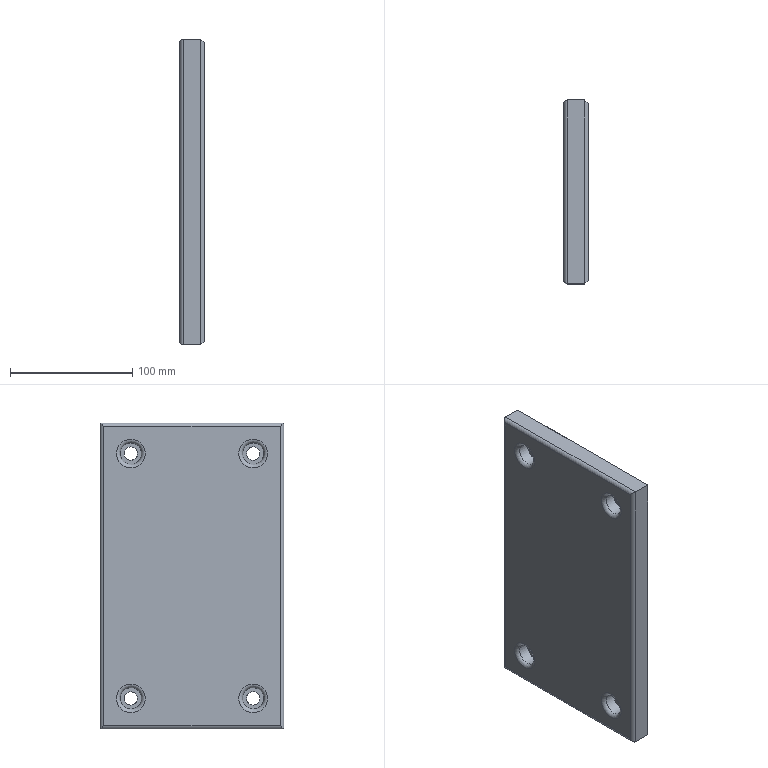Part | NX | features MAIN_BODY 2 | 1 solid | 30 faces | box 20 x 150 x 250 mm | volume 729858 mm3 | plane 14 | cylinder 12 | torus 4 | commonest cylinder face diameters 6 x4 11 x4 17.5 x4
STEP:
#1=CARTESIAN_POINT('',(-1150.,-208.,32.));
#2=VERTEX_POINT('',#1);
#3=CARTESIAN_POINT('',(-1150.,-208.,-212.));
#4=VERTEX_POINT('',#3);
#5=CARTESIAN_POINT('',(-1150.,-208.,-215.));
#6=DIRECTION('',(0.,0.,1.));
#7=VECTOR('',#6,1000.);
#8=LINE('',#5,#7);
#9=EDGE_CURVE('',#2,#4,#8,.F.);
#10=ORIENTED_EDGE('',*,*,#9,.T.);
#11=CARTESIAN_POINT('',(-1150.,-352.,-212.));
#12=VERTEX_POINT('',#11);
#13=CARTESIAN_POINT('',(-1150.,-355.,-212.));
#14=DIRECTION('',(0.,1.,0.));
#15=VECTOR('',#14,1000.);
#16=LINE('',#13,#15);
#17=EDGE_CURVE('',#4,#12,#16,.F.);
#18=ORIENTED_EDGE('',*,*,#17,.T.);
#19=CARTESIAN_POINT('',(-1150.,-352.,32.));
#20=VERTEX_POINT('',#19);
#21=CARTESIAN_POINT('',(-1150.,-352.,35.));
#22=DIRECTION('',(0.,0.,-1.));
#23=VECTOR('',#22,1000.);
#24=LINE('',#21,#23);
#25=EDGE_CURVE('',#12,#20,#24,.F.);
#26=ORIENTED_EDGE('',*,*,#25,.T.);
#27=CARTESIAN_POINT('',(-1150.,-205.,32.));
#28=DIRECTION('',(0.,-1.,0.));
#29=VECTOR('',#28,1000.);
#30=LINE('',#27,#29);
#31=EDGE_CURVE('',#20,#2,#30,.F.);
#32=ORIENTED_EDGE('',*,*,#31,.T.);
#33=EDGE_LOOP('',(#10,#18,#26,#32));
#34=FACE_BOUND('',#33,.T.);
#35=CARTESIAN_POINT('',(-1150.,-230.,-178.25));
#36=VERTEX_POINT('',#35);
#37=CARTESIAN_POINT('',(-1150.,-230.,-190.));
#38=DIRECTION('',(1.,0.,0.));
#39=DIRECTION('',(0.,0.,1.));
#40=AXIS2_PLACEMENT_3D('',#37,#38,#39);
#41=CIRCLE('',#40,11.75);
#42=EDGE_CURVE('',#36,#36,#41,.T.);
#43=ORIENTED_EDGE('',*,*,#42,.T.);
#44=EDGE_LOOP('',(#43));
#45=FACE_BOUND('',#44,.T.);
#46=CARTESIAN_POINT('',(-1150.,-330.,-178.25));
#47=VERTEX_POINT('',#46);
#48=CARTESIAN_POINT('',(-1150.,-330.,-190.));
#49=DIRECTION('',(1.,0.,0.));
#50=DIRECTION('',(0.,0.,1.));
#51=AXIS2_PLACEMENT_3D('',#48,#49,#50);
#52=CIRCLE('',#51,11.75);
#53=EDGE_CURVE('',#47,#47,#52,.T.);
#54=ORIENTED_EDGE('',*,*,#53,.T.);
#55=EDGE_LOOP('',(#54));
#56=FACE_BOUND('',#55,.T.);
#57=CARTESIAN_POINT('',(-1150.,-330.,21.75));
#58=VERTEX_POINT('',#57);
#59=CARTESIAN_POINT('',(-1150.,-330.,10.));
#60=DIRECTION('',(1.,0.,0.));
#61=DIRECTION('',(0.,0.,1.));
#62=AXIS2_PLACEMENT_3D('',#59,#60,#61);
#63=CIRCLE('',#62,11.75);
#64=EDGE_CURVE('',#58,#58,#63,.T.);
#65=ORIENTED_EDGE('',*,*,#64,.T.);
#66=EDGE_LOOP('',(#65));
#67=FACE_BOUND('',#66,.T.);
#68=CARTESIAN_POINT('',(-1150.,-230.,21.75));
#69=VERTEX_POINT('',#68);
#70=CARTESIAN_POINT('',(-1150.,-230.,10.));
#71=DIRECTION('',(1.,0.,0.));
#72=DIRECTION('',(0.,0.,1.));
#73=AXIS2_PLACEMENT_3D('',#70,#71,#72);
#74=CIRCLE('',#73,11.75);
#75=EDGE_CURVE('',#69,#69,#74,.T.);
#76=ORIENTED_EDGE('',*,*,#75,.T.);
#77=EDGE_LOOP('',(#76));
#78=FACE_BOUND('',#77,.T.);
#79=CARTESIAN_POINT('',(-1150.,-205.,35.));
#80=DIRECTION('',(1.,0.,0.));
#81=DIRECTION('',(0.,0.,1.));
#82=AXIS2_PLACEMENT_3D('',#79,#80,#81);
#83=PLANE('',#82);
#84=ADVANCED_FACE('',(#34,#45,#56,#67,#78),#83,.F.);
#85=CARTESIAN_POINT('',(-1130.,-324.5,10.));
#86=VERTEX_POINT('',#85);
#87=CARTESIAN_POINT('',(-1130.,-330.,10.));
#88=DIRECTION('',(-1.,0.,0.));
#89=DIRECTION('',(0.,1.,0.));
#90=AXIS2_PLACEMENT_3D('',#87,#88,#89);
#91=CIRCLE('',#90,5.5);
#92=EDGE_CURVE('',#86,#86,#91,.T.);
#93=ORIENTED_EDGE('',*,*,#92,.F.);
#94=EDGE_LOOP('',(#93));
#95=FACE_BOUND('',#94,.T.);
#96=CARTESIAN_POINT('',(-1138.,-330.,4.5));
#97=VERTEX_POINT('',#96);
#98=CARTESIAN_POINT('',(-1138.,-330.,10.));
#99=DIRECTION('',(-1.,0.,0.));
#100=DIRECTION('',(0.,0.,-1.));
#101=AXIS2_PLACEMENT_3D('',#98,#99,#100);
#102=CIRCLE('',#101,5.5);
#103=EDGE_CURVE('',#97,#97,#102,.T.);
#104=ORIENTED_EDGE('',*,*,#103,.T.);
#105=EDGE_LOOP('',(#104));
#106=FACE_BOUND('',#105,.T.);
#107=CARTESIAN_POINT('',(-1150.,-330.,10.));
#108=DIRECTION('',(1.,0.,0.));
#109=DIRECTION('',(0.,0.,1.));
#110=AXIS2_PLACEMENT_3D('',#107,#108,#109);
#111=CYLINDRICAL_SURFACE('',#110,5.5);
#112=ADVANCED_FACE('',(#95,#106),#111,.F.);
#113=CARTESIAN_POINT('',(-1130.,-235.5,-190.));
#114=VERTEX_POINT('',#113);
#115=CARTESIAN_POINT('',(-1130.,-230.,-190.));
#116=DIRECTION('',(-1.,0.,0.));
#117=DIRECTION('',(0.,-1.,0.));
#118=AXIS2_PLACEMENT_3D('',#115,#116,#117);
#119=CIRCLE('',#118,5.5);
#120=EDGE_CURVE('',#114,#114,#119,.T.);
#121=ORIENTED_EDGE('',*,*,#120,.F.);
#122=EDGE_LOOP('',(#121));
#123=FACE_BOUND('',#122,.T.);
#124=CARTESIAN_POINT('',(-1138.,-230.,-195.5));
#125=VERTEX_POINT('',#124);
#126=CARTESIAN_POINT('',(-1138.,-230.,-190.));
#127=DIRECTION('',(-1.,0.,0.));
#128=DIRECTION('',(0.,0.,-1.));
#129=AXIS2_PLACEMENT_3D('',#126,#127,#128);
#130=CIRCLE('',#129,5.5);
#131=EDGE_CURVE('',#125,#125,#130,.T.);
#132=ORIENTED_EDGE('',*,*,#131,.T.);
#133=EDGE_LOOP('',(#132));
#134=FACE_BOUND('',#133,.T.);
#135=CARTESIAN_POINT('',(-1150.,-230.,-190.));
#136=DIRECTION('',(1.,0.,0.));
#137=DIRECTION('',(0.,0.,1.));
#138=AXIS2_PLACEMENT_3D('',#135,#136,#137);
#139=CYLINDRICAL_SURFACE('',#138,5.5);
#140=ADVANCED_FACE('',(#123,#134),#139,.F.);
#141=CARTESIAN_POINT('',(-1130.,-352.,32.));
#142=VERTEX_POINT('',#141);
#143=CARTESIAN_POINT('',(-1130.,-352.,-212.));
#144=VERTEX_POINT('',#143);
#145=CARTESIAN_POINT('',(-1130.,-352.,35.));
#146=DIRECTION('',(0.,0.,-1.));
#147=VECTOR('',#146,1000.);
#148=LINE('',#145,#147);
#149=EDGE_CURVE('',#142,#144,#148,.T.);
#150=ORIENTED_EDGE('',*,*,#149,.T.);
#151=CARTESIAN_POINT('',(-1130.,-208.,-212.));
#152=VERTEX_POINT('',#151);
#153=CARTESIAN_POINT('',(-1130.,-205.,-212.));
#154=DIRECTION('',(0.,1.,0.));
#155=VECTOR('',#154,1000.);
#156=LINE('',#153,#155);
#157=EDGE_CURVE('',#144,#152,#156,.T.);
#158=ORIENTED_EDGE('',*,*,#157,.T.);
#159=CARTESIAN_POINT('',(-1130.,-208.,32.));
#160=VERTEX_POINT('',#159);
#161=CARTESIAN_POINT('',(-1130.,-208.,35.));
#162=DIRECTION('',(0.,0.,1.));
#163=VECTOR('',#162,1000.);
#164=LINE('',#161,#163);
#165=EDGE_CURVE('',#152,#160,#164,.T.);
#166=ORIENTED_EDGE('',*,*,#165,.T.);
#167=CARTESIAN_POINT('',(-1130.,-205.,32.));
#168=DIRECTION('',(0.,-1.,0.));
#169=VECTOR('',#168,1000.);
#170=LINE('',#167,#169);
#171=EDGE_CURVE('',#160,#142,#170,.T.);
#172=ORIENTED_EDGE('',*,*,#171,.T.);
#173=EDGE_LOOP('',(#150,#158,#166,#172));
#174=FACE_BOUND('',#173,.T.);
#175=CARTESIAN_POINT('',(-1130.,-235.5,10.));
#176=VERTEX_POINT('',#175);
#177=CARTESIAN_POINT('',(-1130.,-230.,10.));
#178=DIRECTION('',(1.,0.,0.));
#179=DIRECTION('',(0.,-1.,0.));
#180=AXIS2_PLACEMENT_3D('',#177,#178,#179);
#181=CIRCLE('',#180,5.5);
#182=EDGE_CURVE('',#176,#176,#181,.T.);
#183=ORIENTED_EDGE('',*,*,#182,.F.);
#184=EDGE_LOOP('',(#183));
#185=FACE_BOUND('',#184,.T.);
#186=ORIENTED_EDGE('',*,*,#92,.T.);
#187=EDGE_LOOP('',(#186));
#188=FACE_BOUND('',#187,.T.);
#189=CARTESIAN_POINT('',(-1130.,-324.5,-190.));
#190=VERTEX_POINT('',#189);
#191=CARTESIAN_POINT('',(-1130.,-330.,-190.));
#192=DIRECTION('',(1.,0.,0.));
#193=DIRECTION('',(0.,1.,0.));
#194=AXIS2_PLACEMENT_3D('',#191,#192,#193);
#195=CIRCLE('',#194,5.5);
#196=EDGE_CURVE('',#190,#190,#195,.T.);
#197=ORIENTED_EDGE('',*,*,#196,.F.);
#198=EDGE_LOOP('',(#197));
#199=FACE_BOUND('',#198,.T.);
#200=ORIENTED_EDGE('',*,*,#120,.T.);
#201=EDGE_LOOP('',(#200));
#202=FACE_BOUND('',#201,.T.);
#203=CARTESIAN_POINT('',(-1130.,-205.,35.));
#204=DIRECTION('',(1.,0.,0.));
#205=DIRECTION('',(0.,0.,1.));
#206=AXIS2_PLACEMENT_3D('',#203,#204,#205);
#207=PLANE('',#206);
#208=ADVANCED_FACE('',(#174,#185,#188,#199,#202),#207,.T.);
#209=CARTESIAN_POINT('',(-1147.,-205.,35.));
#210=VERTEX_POINT('',#209);
#211=CARTESIAN_POINT('',(-1133.,-205.,35.));
#212=VERTEX_POINT('',#211);
#213=CARTESIAN_POINT('',(-1150.,-205.,35.));
#214=DIRECTION('',(1.,0.,0.));
#215=VECTOR('',#214,1000.);
#216=LINE('',#213,#215);
#217=EDGE_CURVE('',#210,#212,#216,.T.);
#218=ORIENTED_EDGE('',*,*,#217,.T.);
#219=CARTESIAN_POINT('',(-1133.,-205.,-215.));
#220=VERTEX_POINT('',#219);
#221=CARTESIAN_POINT('',(-1133.,-205.,-215.));
#222=DIRECTION('',(0.,0.,-1.));
#223=VECTOR('',#222,1000.);
#224=LINE('',#221,#223);
#225=EDGE_CURVE('',#212,#220,#224,.T.);
#226=ORIENTED_EDGE('',*,*,#225,.T.);
#227=CARTESIAN_POINT('',(-1147.,-205.,-215.));
#228=VERTEX_POINT('',#227);
#229=CARTESIAN_POINT('',(-1150.,-205.,-215.));
#230=DIRECTION('',(1.,0.,0.));
#231=VECTOR('',#230,1000.);
#232=LINE('',#229,#231);
#233=EDGE_CURVE('',#228,#220,#232,.T.);
#234=ORIENTED_EDGE('',*,*,#233,.F.);
#235=CARTESIAN_POINT('',(-1147.,-205.,35.));
#236=DIRECTION('',(0.,0.,1.));
#237=VECTOR('',#236,1000.);
#238=LINE('',#235,#237);
#239=EDGE_CURVE('',#228,#210,#238,.T.);
#240=ORIENTED_EDGE('',*,*,#239,.T.);
#241=EDGE_LOOP('',(#218,#226,#234,#240));
#242=FACE_BOUND('',#241,.T.);
#243=CARTESIAN_POINT('',(-1150.,-205.,-215.));
#244=DIRECTION('',(0.,1.,0.));
#245=DIRECTION('',(0.,0.,-1.));
#246=AXIS2_PLACEMENT_3D('',#243,#244,#245);
#247=PLANE('',#246);
#248=ADVANCED_FACE('',(#242),#247,.T.);
#249=CARTESIAN_POINT('',(-1147.,-355.,35.));
#250=VERTEX_POINT('',#249);
#251=CARTESIAN_POINT('',(-1133.,-355.,35.));
#252=VERTEX_POINT('',#251);
#253=CARTESIAN_POINT('',(-1150.,-355.,35.));
#254=DIRECTION('',(1.,0.,0.));
#255=VECTOR('',#254,1000.);
#256=LINE('',#253,#255);
#257=EDGE_CURVE('',#250,#252,#256,.T.);
#258=ORIENTED_EDGE('',*,*,#257,.T.);
#259=CARTESIAN_POINT('',(-1133.,-205.,35.));
#260=DIRECTION('',(0.,1.,0.));
#261=VECTOR('',#260,1000.);
#262=LINE('',#259,#261);
#263=EDGE_CURVE('',#252,#212,#262,.T.);
#264=ORIENTED_EDGE('',*,*,#263,.T.);
#265=ORIENTED_EDGE('',*,*,#217,.F.);
#266=CARTESIAN_POINT('',(-1147.,-355.,35.));
#267=DIRECTION('',(0.,-1.,0.));
#268=VECTOR('',#267,1000.);
#269=LINE('',#266,#268);
#270=EDGE_CURVE('',#210,#250,#269,.T.);
#271=ORIENTED_EDGE('',*,*,#270,.T.);
#272=EDGE_LOOP('',(#258,#264,#265,#271));
#273=FACE_BOUND('',#272,.T.);
#274=CARTESIAN_POINT('',(-1150.,-205.,35.));
#275=DIRECTION('',(0.,0.,1.));
#276=DIRECTION('',(0.,1.,0.));
#277=AXIS2_PLACEMENT_3D('',#274,#275,#276);
#278=PLANE('',#277);
#279=ADVANCED_FACE('',(#273),#278,.T.);
#280=CARTESIAN_POINT('',(-1147.,-355.,-215.));
#281=VERTEX_POINT('',#280);
#282=CARTESIAN_POINT('',(-1133.,-355.,-215.));
#283=VERTEX_POINT('',#282);
#284=CARTESIAN_POINT('',(-1150.,-355.,-215.));
#285=DIRECTION('',(1.,0.,0.));
#286=VECTOR('',#285,1000.);
#287=LINE('',#284,#286);
#288=EDGE_CURVE('',#281,#283,#287,.T.);
#289=ORIENTED_EDGE('',*,*,#288,.T.);
#290=CARTESIAN_POINT('',(-1133.,-355.,35.));
#291=DIRECTION('',(0.,0.,1.));
#292=VECTOR('',#291,1000.);
#293=LINE('',#290,#292);
#294=EDGE_CURVE('',#283,#252,#293,.T.);
#295=ORIENTED_EDGE('',*,*,#294,.T.);
#296=ORIENTED_EDGE('',*,*,#257,.F.);
#297=CARTESIAN_POINT('',(-1147.,-355.,-215.));
#298=DIRECTION('',(0.,0.,-1.));
#299=VECTOR('',#298,1000.);
#300=LINE('',#297,#299);
#301=EDGE_CURVE('',#250,#281,#300,.T.);
#302=ORIENTED_EDGE('',*,*,#301,.T.);
#303=EDGE_LOOP('',(#289,#295,#296,#302));
#304=FACE_BOUND('',#303,.T.);
#305=CARTESIAN_POINT('',(-1150.,-355.,35.));
#306=DIRECTION('',(0.,-1.,0.));
#307=DIRECTION('',(0.,0.,1.));
#308=AXIS2_PLACEMENT_3D('',#305,#306,#307);
#309=PLANE('',#308);
#310=ADVANCED_FACE('',(#304),#309,.T.);
#311=ORIENTED_EDGE('',*,*,#233,.T.);
#312=CARTESIAN_POINT('',(-1133.,-355.,-215.));
#313=DIRECTION('',(0.,-1.,0.));
#314=VECTOR('',#313,1000.);
#315=LINE('',#312,#314);
#316=EDGE_CURVE('',#220,#283,#315,.T.);
#317=ORIENTED_EDGE('',*,*,#316,.T.);
#318=ORIENTED_EDGE('',*,*,#288,.F.);
#319=CARTESIAN_POINT('',(-1147.,-205.,-215.));
#320=DIRECTION('',(0.,1.,0.));
#321=VECTOR('',#320,1000.);
#322=LINE('',#319,#321);
#323=EDGE_CURVE('',#281,#228,#322,.T.);
#324=ORIENTED_EDGE('',*,*,#323,.T.);
#325=EDGE_LOOP('',(#311,#317,#318,#324));
#326=FACE_BOUND('',#325,.T.);
#327=CARTESIAN_POINT('',(-1150.,-355.,-215.));
#328=DIRECTION('',(0.,0.,-1.));
#329=DIRECTION('',(0.,-1.,0.));
#330=AXIS2_PLACEMENT_3D('',#327,#328,#329);
#331=PLANE('',#330);
#332=ADVANCED_FACE('',(#326),#331,.T.);
#333=CARTESIAN_POINT('',(-1138.,-330.,-184.5));
#334=VERTEX_POINT('',#333);
#335=CARTESIAN_POINT('',(-1138.,-330.,-190.));
#336=DIRECTION('',(1.,0.,0.));
#337=DIRECTION('',(0.,0.,1.));
#338=AXIS2_PLACEMENT_3D('',#335,#336,#337);
#339=CIRCLE('',#338,5.5);
#340=EDGE_CURVE('',#334,#334,#339,.F.);
#341=ORIENTED_EDGE('',*,*,#340,.T.);
#342=EDGE_LOOP('',(#341));
#343=FACE_BOUND('',#342,.T.);
#344=ORIENTED_EDGE('',*,*,#196,.T.);
#345=EDGE_LOOP('',(#344));
#346=FACE_BOUND('',#345,.T.);
#347=CARTESIAN_POINT('',(-1150.,-330.,-190.));
#348=DIRECTION('',(1.,0.,0.));
#349=DIRECTION('',(0.,0.,1.));
#350=AXIS2_PLACEMENT_3D('',#347,#348,#349);
#351=CYLINDRICAL_SURFACE('',#350,5.5);
#352=ADVANCED_FACE('',(#343,#346),#351,.F.);
#353=CARTESIAN_POINT('',(-1138.,-230.,15.5));
#354=VERTEX_POINT('',#353);
#355=CARTESIAN_POINT('',(-1138.,-230.,10.));
#356=DIRECTION('',(1.,0.,0.));
#357=DIRECTION('',(0.,0.,1.));
#358=AXIS2_PLACEMENT_3D('',#355,#356,#357);
#359=CIRCLE('',#358,5.5);
#360=EDGE_CURVE('',#354,#354,#359,.F.);
#361=ORIENTED_EDGE('',*,*,#360,.T.);
#362=EDGE_LOOP('',(#361));
#363=FACE_BOUND('',#362,.T.);
#364=ORIENTED_EDGE('',*,*,#182,.T.);
#365=EDGE_LOOP('',(#364));
#366=FACE_BOUND('',#365,.T.);
#367=CARTESIAN_POINT('',(-1150.,-230.,10.));
#368=DIRECTION('',(1.,0.,0.));
#369=DIRECTION('',(0.,0.,1.));
#370=AXIS2_PLACEMENT_3D('',#367,#368,#369);
#371=CYLINDRICAL_SURFACE('',#370,5.5);
#372=ADVANCED_FACE('',(#363,#366),#371,.F.);
#373=CARTESIAN_POINT('',(-1147.,-230.,-181.25));
#374=VERTEX_POINT('',#373);
#375=CARTESIAN_POINT('',(-1147.,-230.,-190.));
#376=DIRECTION('',(1.,0.,0.));
#377=DIRECTION('',(0.,0.,1.));
#378=AXIS2_PLACEMENT_3D('',#375,#376,#377);
#379=CIRCLE('',#378,8.75);
#380=EDGE_CURVE('',#374,#374,#379,.F.);
#381=ORIENTED_EDGE('',*,*,#380,.T.);
#382=EDGE_LOOP('',(#381));
#383=FACE_BOUND('',#382,.T.);
#384=CARTESIAN_POINT('',(-1138.,-238.75,-190.));
#385=VERTEX_POINT('',#384);
#386=CARTESIAN_POINT('',(-1138.,-230.,-190.));
#387=DIRECTION('',(-1.,0.,0.));
#388=DIRECTION('',(0.,-1.,0.));
#389=AXIS2_PLACEMENT_3D('',#386,#387,#388);
#390=CIRCLE('',#389,8.75);
#391=EDGE_CURVE('',#385,#385,#390,.T.);
#392=ORIENTED_EDGE('',*,*,#391,.F.);
#393=EDGE_LOOP('',(#392));
#394=FACE_BOUND('',#393,.T.);
#395=CARTESIAN_POINT('',(-1160.,-230.,-190.));
#396=DIRECTION('',(1.,0.,0.));
#397=DIRECTION('',(0.,0.,1.));
#398=AXIS2_PLACEMENT_3D('',#395,#396,#397);
#399=CYLINDRICAL_SURFACE('',#398,8.75);
#400=ADVANCED_FACE('',(#383,#394),#399,.F.);
#401=ORIENTED_EDGE('',*,*,#131,.F.);
#402=EDGE_LOOP('',(#401));
#403=FACE_BOUND('',#402,.T.);
#404=ORIENTED_EDGE('',*,*,#391,.T.);
#405=EDGE_LOOP('',(#404));
#406=FACE_BOUND('',#405,.T.);
#407=CARTESIAN_POINT('',(-1138.,-230.,-190.));
#408=DIRECTION('',(-1.,0.,0.));
#409=DIRECTION('',(0.,0.,-1.));
#410=AXIS2_PLACEMENT_3D('',#407,#408,#409);
#411=PLANE('',#410);
#412=ADVANCED_FACE('',(#403,#406),#411,.T.);
#413=CARTESIAN_POINT('',(-1147.,-230.,18.75));
#414=VERTEX_POINT('',#413);
#415=CARTESIAN_POINT('',(-1147.,-230.,10.));
#416=DIRECTION('',(1.,0.,0.));
#417=DIRECTION('',(0.,0.,1.));
#418=AXIS2_PLACEMENT_3D('',#415,#416,#417);
#419=CIRCLE('',#418,8.75);
#420=EDGE_CURVE('',#414,#414,#419,.F.);
#421=ORIENTED_EDGE('',*,*,#420,.T.);
#422=EDGE_LOOP('',(#421));
#423=FACE_BOUND('',#422,.T.);
#424=CARTESIAN_POINT('',(-1138.,-238.75,10.));
#425=VERTEX_POINT('',#424);
#426=CARTESIAN_POINT('',(-1138.,-230.,10.));
#427=DIRECTION('',(1.,0.,0.));
#428=DIRECTION('',(0.,-1.,0.));
#429=AXIS2_PLACEMENT_3D('',#426,#427,#428);
#430=CIRCLE('',#429,8.75);
#431=EDGE_CURVE('',#425,#425,#430,.T.);
#432=ORIENTED_EDGE('',*,*,#431,.T.);
#433=EDGE_LOOP('',(#432));
#434=FACE_BOUND('',#433,.T.);
#435=CARTESIAN_POINT('',(-1160.,-230.,10.));
#436=DIRECTION('',(1.,0.,0.));
#437=DIRECTION('',(0.,0.,1.));
#438=AXIS2_PLACEMENT_3D('',#435,#436,#437);
#439=CYLINDRICAL_SURFACE('',#438,8.75);
#440=ADVANCED_FACE('',(#423,#434),#439,.F.);
#441=ORIENTED_EDGE('',*,*,#431,.F.);
#442=EDGE_LOOP('',(#441));
#443=FACE_BOUND('',#442,.T.);
#444=ORIENTED_EDGE('',*,*,#360,.F.);
#445=EDGE_LOOP('',(#444));
#446=FACE_BOUND('',#445,.T.);
#447=CARTESIAN_POINT('',(-1138.,-230.,10.));
#448=DIRECTION('',(1.,0.,0.));
#449=DIRECTION('',(0.,0.,1.));
#450=AXIS2_PLACEMENT_3D('',#447,#448,#449);
#451=PLANE('',#450);
#452=ADVANCED_FACE('',(#443,#446),#451,.F.);
#453=CARTESIAN_POINT('',(-1147.,-330.,-181.25));
#454=VERTEX_POINT('',#453);
#455=CARTESIAN_POINT('',(-1147.,-330.,-190.));
#456=DIRECTION('',(1.,0.,0.));
#457=DIRECTION('',(0.,0.,1.));
#458=AXIS2_PLACEMENT_3D('',#455,#456,#457);
#459=CIRCLE('',#458,8.75);
#460=EDGE_CURVE('',#454,#454,#459,.F.);
#461=ORIENTED_EDGE('',*,*,#460,.T.);
#462=EDGE_LOOP('',(#461));
#463=FACE_BOUND('',#462,.T.);
#464=CARTESIAN_POINT('',(-1138.,-321.25,-190.));
#465=VERTEX_POINT('',#464);
#466=CARTESIAN_POINT('',(-1138.,-330.,-190.));
#467=DIRECTION('',(1.,0.,0.));
#468=DIRECTION('',(0.,1.,0.));
#469=AXIS2_PLACEMENT_3D('',#466,#467,#468);
#470=CIRCLE('',#469,8.75);
#471=EDGE_CURVE('',#465,#465,#470,.T.);
#472=ORIENTED_EDGE('',*,*,#471,.T.);
#473=EDGE_LOOP('',(#472));
#474=FACE_BOUND('',#473,.T.);
#475=CARTESIAN_POINT('',(-1160.,-330.,-190.));
#476=DIRECTION('',(1.,0.,0.));
#477=DIRECTION('',(0.,0.,1.));
#478=AXIS2_PLACEMENT_3D('',#475,#476,#477);
#479=CYLINDRICAL_SURFACE('',#478,8.75);
#480=ADVANCED_FACE('',(#463,#474),#479,.F.);
#481=ORIENTED_EDGE('',*,*,#471,.F.);
#482=EDGE_LOOP('',(#481));
#483=FACE_BOUND('',#482,.T.);
#484=ORIENTED_EDGE('',*,*,#340,.F.);
#485=EDGE_LOOP('',(#484));
#486=FACE_BOUND('',#485,.T.);
#487=CARTESIAN_POINT('',(-1138.,-330.,-190.));
#488=DIRECTION('',(1.,0.,0.));
#489=DIRECTION('',(0.,0.,1.));
#490=AXIS2_PLACEMENT_3D('',#487,#488,#489);
#491=PLANE('',#490);
#492=ADVANCED_FACE('',(#483,#486),#491,.F.);
#493=CARTESIAN_POINT('',(-1147.,-330.,18.75));
#494=VERTEX_POINT('',#493);
#495=CARTESIAN_POINT('',(-1147.,-330.,10.));
#496=DIRECTION('',(1.,0.,0.));
#497=DIRECTION('',(0.,0.,1.));
#498=AXIS2_PLACEMENT_3D('',#495,#496,#497);
#499=CIRCLE('',#498,8.75);
#500=EDGE_CURVE('',#494,#494,#499,.F.);
#501=ORIENTED_EDGE('',*,*,#500,.T.);
#502=EDGE_LOOP('',(#501));
#503=FACE_BOUND('',#502,.T.);
#504=CARTESIAN_POINT('',(-1138.,-321.25,10.));
#505=VERTEX_POINT('',#504);
#506=CARTESIAN_POINT('',(-1138.,-330.,10.));
#507=DIRECTION('',(-1.,0.,0.));
#508=DIRECTION('',(0.,1.,0.));
#509=AXIS2_PLACEMENT_3D('',#506,#507,#508);
#510=CIRCLE('',#509,8.75);
#511=EDGE_CURVE('',#505,#505,#510,.T.);
#512=ORIENTED_EDGE('',*,*,#511,.F.);
#513=EDGE_LOOP('',(#512));
#514=FACE_BOUND('',#513,.T.);
#515=CARTESIAN_POINT('',(-1160.,-330.,10.));
#516=DIRECTION('',(1.,0.,0.));
#517=DIRECTION('',(0.,0.,1.));
#518=AXIS2_PLACEMENT_3D('',#515,#516,#517);
#519=CYLINDRICAL_SURFACE('',#518,8.75);
#520=ADVANCED_FACE('',(#503,#514),#519,.F.);
#521=ORIENTED_EDGE('',*,*,#103,.F.);
#522=EDGE_LOOP('',(#521));
#523=FACE_BOUND('',#522,.T.);
#524=ORIENTED_EDGE('',*,*,#511,.T.);
#525=EDGE_LOOP('',(#524));
#526=FACE_BOUND('',#525,.T.);
#527=CARTESIAN_POINT('',(-1138.,-330.,10.));
#528=DIRECTION('',(-1.,0.,0.));
#529=DIRECTION('',(0.,0.,-1.));
#530=AXIS2_PLACEMENT_3D('',#527,#528,#529);
#531=PLANE('',#530);
#532=ADVANCED_FACE('',(#523,#526),#531,.T.);
#533=CARTESIAN_POINT('',(-1147.,-208.,32.));
#534=DIRECTION('',(0.,0.7071,-0.7071));
#535=DIRECTION('',(0.,0.7071,0.7071));
#536=AXIS2_PLACEMENT_3D('',#533,#534,#535);
#537=ELLIPSE('',#536,4.243,3.);
#538=EDGE_CURVE('',#2,#210,#537,.T.);
#539=ORIENTED_EDGE('',*,*,#538,.F.);
#540=ORIENTED_EDGE('',*,*,#31,.F.);
#541=CARTESIAN_POINT('',(-1147.,-352.,32.));
#542=DIRECTION('',(0.,0.7071,0.7071));
#543=DIRECTION('',(0.,0.7071,-0.7071));
#544=AXIS2_PLACEMENT_3D('',#541,#542,#543);
#545=ELLIPSE('',#544,4.243,3.);
#546=EDGE_CURVE('',#250,#20,#545,.F.);
#547=ORIENTED_EDGE('',*,*,#546,.F.);
#548=ORIENTED_EDGE('',*,*,#270,.F.);
#549=EDGE_LOOP('',(#539,#540,#547,#548));
#550=FACE_BOUND('',#549,.T.);
#551=CARTESIAN_POINT('',(-1147.,-205.,32.));
#552=DIRECTION('',(0.,1.,0.));
#553=DIRECTION('',(0.,0.,-1.));
#554=AXIS2_PLACEMENT_3D('',#551,#552,#553);
#555=CYLINDRICAL_SURFACE('',#554,3.);
#556=ADVANCED_FACE('',(#550),#555,.T.);
#557=ORIENTED_EDGE('',*,*,#546,.T.);
#558=ORIENTED_EDGE('',*,*,#25,.F.);
#559=CARTESIAN_POINT('',(-1147.,-352.,-212.));
#560=DIRECTION('',(0.,-0.7071,0.7071));
#561=DIRECTION('',(0.,0.7071,0.7071));
#562=AXIS2_PLACEMENT_3D('',#559,#560,#561);
#563=ELLIPSE('',#562,4.243,3.);
#564=EDGE_CURVE('',#281,#12,#563,.F.);
#565=ORIENTED_EDGE('',*,*,#564,.F.);
#566=ORIENTED_EDGE('',*,*,#301,.F.);
#567=EDGE_LOOP('',(#557,#558,#565,#566));
#568=FACE_BOUND('',#567,.T.);
#569=CARTESIAN_POINT('',(-1147.,-352.,35.));
#570=DIRECTION('',(0.,0.,1.));
#571=DIRECTION('',(0.,1.,0.));
#572=AXIS2_PLACEMENT_3D('',#569,#570,#571);
#573=CYLINDRICAL_SURFACE('',#572,3.);
#574=ADVANCED_FACE('',(#568),#573,.T.);
#575=ORIENTED_EDGE('',*,*,#538,.T.);
#576=ORIENTED_EDGE('',*,*,#239,.F.);
#577=CARTESIAN_POINT('',(-1147.,-208.,-212.));
#578=DIRECTION('',(0.,-0.7071,-0.7071));
#579=DIRECTION('',(0.,0.7071,-0.7071));
#580=AXIS2_PLACEMENT_3D('',#577,#578,#579);
#581=ELLIPSE('',#580,4.243,3.);
#582=EDGE_CURVE('',#4,#228,#581,.T.);
#583=ORIENTED_EDGE('',*,*,#582,.F.);
#584=ORIENTED_EDGE('',*,*,#9,.F.);
#585=EDGE_LOOP('',(#575,#576,#583,#584));
#586=FACE_BOUND('',#585,.T.);
#587=CARTESIAN_POINT('',(-1147.,-208.,-215.));
#588=DIRECTION('',(0.,0.,-1.));
#589=DIRECTION('',(0.,-1.,0.));
#590=AXIS2_PLACEMENT_3D('',#587,#588,#589);
#591=CYLINDRICAL_SURFACE('',#590,3.);
#592=ADVANCED_FACE('',(#586),#591,.T.);
#593=ORIENTED_EDGE('',*,*,#564,.T.);
#594=ORIENTED_EDGE('',*,*,#17,.F.);
#595=ORIENTED_EDGE('',*,*,#582,.T.);
#596=ORIENTED_EDGE('',*,*,#323,.F.);
#597=EDGE_LOOP('',(#593,#594,#595,#596));
#598=FACE_BOUND('',#597,.T.);
#599=CARTESIAN_POINT('',(-1147.,-355.,-212.));
#600=DIRECTION('',(0.,-1.,0.));
#601=DIRECTION('',(0.,0.,1.));
#602=AXIS2_PLACEMENT_3D('',#599,#600,#601);
#603=CYLINDRICAL_SURFACE('',#602,3.);
#604=ADVANCED_FACE('',(#598),#603,.T.);
#605=ORIENTED_EDGE('',*,*,#42,.F.);
#606=EDGE_LOOP('',(#605));
#607=FACE_BOUND('',#606,.T.);
#608=ORIENTED_EDGE('',*,*,#380,.F.);
#609=EDGE_LOOP('',(#608));
#610=FACE_BOUND('',#609,.T.);
#611=CARTESIAN_POINT('',(-1147.,-230.,-190.));
#612=DIRECTION('',(1.,0.,0.));
#613=DIRECTION('',(0.,0.,1.));
#614=AXIS2_PLACEMENT_3D('',#611,#612,#613);
#615=TOROIDAL_SURFACE('',#614,11.75,3.);
#616=ADVANCED_FACE('',(#607,#610),#615,.T.);
#617=ORIENTED_EDGE('',*,*,#460,.F.);
#618=EDGE_LOOP('',(#617));
#619=FACE_BOUND('',#618,.T.);
#620=ORIENTED_EDGE('',*,*,#53,.F.);
#621=EDGE_LOOP('',(#620));
#622=FACE_BOUND('',#621,.T.);
#623=CARTESIAN_POINT('',(-1147.,-330.,-190.));
#624=DIRECTION('',(1.,0.,0.));
#625=DIRECTION('',(0.,0.,1.));
#626=AXIS2_PLACEMENT_3D('',#623,#624,#625);
#627=TOROIDAL_SURFACE('',#626,11.75,3.);
#628=ADVANCED_FACE('',(#619,#622),#627,.T.);
#629=ORIENTED_EDGE('',*,*,#64,.F.);
#630=EDGE_LOOP('',(#629));
#631=FACE_BOUND('',#630,.T.);
#632=ORIENTED_EDGE('',*,*,#500,.F.);
#633=EDGE_LOOP('',(#632));
#634=FACE_BOUND('',#633,.T.);
#635=CARTESIAN_POINT('',(-1147.,-330.,10.));
#636=DIRECTION('',(1.,0.,0.));
#637=DIRECTION('',(0.,0.,1.));
#638=AXIS2_PLACEMENT_3D('',#635,#636,#637);
#639=TOROIDAL_SURFACE('',#638,11.75,3.);
#640=ADVANCED_FACE('',(#631,#634),#639,.T.);
#641=ORIENTED_EDGE('',*,*,#420,.F.);
#642=EDGE_LOOP('',(#641));
#643=FACE_BOUND('',#642,.T.);
#644=ORIENTED_EDGE('',*,*,#75,.F.);
#645=EDGE_LOOP('',(#644));
#646=FACE_BOUND('',#645,.T.);
#647=CARTESIAN_POINT('',(-1147.,-230.,10.));
#648=DIRECTION('',(1.,0.,0.));
#649=DIRECTION('',(0.,0.,1.));
#650=AXIS2_PLACEMENT_3D('',#647,#648,#649);
#651=TOROIDAL_SURFACE('',#650,11.75,3.);
#652=ADVANCED_FACE('',(#643,#646),#651,.T.);
#653=CARTESIAN_POINT('',(-1131.,-207.,33.));
#654=DIRECTION('',(-0.5774,0.5774,0.5774));
#655=VECTOR('',#654,1000.);
#656=LINE('',#653,#655);
#657=EDGE_CURVE('',#212,#160,#656,.F.);
#658=ORIENTED_EDGE('',*,*,#657,.F.);
#659=ORIENTED_EDGE('',*,*,#263,.F.);
#660=CARTESIAN_POINT('',(-1131.,-353.,33.));
#661=DIRECTION('',(-0.5774,-0.5774,0.5774));
#662=VECTOR('',#661,1000.);
#663=LINE('',#660,#662);
#664=EDGE_CURVE('',#142,#252,#663,.T.);
#665=ORIENTED_EDGE('',*,*,#664,.F.);
#666=ORIENTED_EDGE('',*,*,#171,.F.);
#667=EDGE_LOOP('',(#658,#659,#665,#666));
#668=FACE_BOUND('',#667,.T.);
#669=CARTESIAN_POINT('',(-1130.,-205.,32.));
#670=DIRECTION('',(-0.7071,0.,-0.7071));
#671=DIRECTION('',(0.7071,0.,-0.7071));
#672=AXIS2_PLACEMENT_3D('',#669,#670,#671);
#673=PLANE('',#672);
#674=ADVANCED_FACE('',(#668),#673,.F.);
#675=ORIENTED_EDGE('',*,*,#664,.T.);
#676=ORIENTED_EDGE('',*,*,#294,.F.);
#677=CARTESIAN_POINT('',(-1047.667,-269.667,-129.667));
#678=DIRECTION('',(0.5774,0.5774,0.5774));
#679=VECTOR('',#678,1000.);
#680=LINE('',#677,#679);
#681=EDGE_CURVE('',#144,#283,#680,.F.);
#682=ORIENTED_EDGE('',*,*,#681,.F.);
#683=ORIENTED_EDGE('',*,*,#149,.F.);
#684=EDGE_LOOP('',(#675,#676,#682,#683));
#685=FACE_BOUND('',#684,.T.);
#686=CARTESIAN_POINT('',(-1130.,-352.,35.));
#687=DIRECTION('',(-0.7071,0.7071,0.));
#688=DIRECTION('',(-0.7071,-0.7071,0.));
#689=AXIS2_PLACEMENT_3D('',#686,#687,#688);
#690=PLANE('',#689);
#691=ADVANCED_FACE('',(#685),#690,.F.);
#692=ORIENTED_EDGE('',*,*,#657,.T.);
#693=ORIENTED_EDGE('',*,*,#165,.F.);
#694=CARTESIAN_POINT('',(-1047.667,-290.333,-129.667));
#695=DIRECTION('',(-0.5774,0.5774,-0.5774));
#696=VECTOR('',#695,1000.);
#697=LINE('',#694,#696);
#698=EDGE_CURVE('',#220,#152,#697,.F.);
#699=ORIENTED_EDGE('',*,*,#698,.F.);
#700=ORIENTED_EDGE('',*,*,#225,.F.);
#701=EDGE_LOOP('',(#692,#693,#699,#700));
#702=FACE_BOUND('',#701,.T.);
#703=CARTESIAN_POINT('',(-1130.,-208.,35.));
#704=DIRECTION('',(-0.7071,-0.7071,0.));
#705=DIRECTION('',(0.7071,-0.7071,0.));
#706=AXIS2_PLACEMENT_3D('',#703,#704,#705);
#707=PLANE('',#706);
#708=ADVANCED_FACE('',(#702),#707,.F.);
#709=ORIENTED_EDGE('',*,*,#681,.T.);
#710=ORIENTED_EDGE('',*,*,#316,.F.);
#711=ORIENTED_EDGE('',*,*,#698,.T.);
#712=ORIENTED_EDGE('',*,*,#157,.F.);
#713=EDGE_LOOP('',(#709,#710,#711,#712));
#714=FACE_BOUND('',#713,.T.);
#715=CARTESIAN_POINT('',(-1130.,-205.,-212.));
#716=DIRECTION('',(-0.7071,0.,0.7071));
#717=DIRECTION('',(-0.7071,0.,-0.7071));
#718=AXIS2_PLACEMENT_3D('',#715,#716,#717);
#719=PLANE('',#718);
#720=ADVANCED_FACE('',(#714),#719,.F.);
#721=CLOSED_SHELL('',(#84,#112,#140,#208,#248,#279,#310,#332,#352,#372,#400,#412,#440,#452,#480,#492,#520,#532,#556,#574,#592,#604,#616,#628,#640,#652,#674,#691,#708,#720));
#722=MANIFOLD_SOLID_BREP('',#721);
#723=(LENGTH_UNIT()NAMED_UNIT(*)SI_UNIT(.MILLI.,.METRE.));
#724=UNCERTAINTY_MEASURE_WITH_UNIT(LENGTH_MEASURE(0.00001),#723,'','');
#725=(NAMED_UNIT(*)PLANE_ANGLE_UNIT()SI_UNIT($,.RADIAN.));
#726=(NAMED_UNIT(*)SI_UNIT($,.STERADIAN.)SOLID_ANGLE_UNIT());
#727=(GEOMETRIC_REPRESENTATION_CONTEXT(3)GLOBAL_UNCERTAINTY_ASSIGNED_CONTEXT((#724))GLOBAL_UNIT_ASSIGNED_CONTEXT((#723,#725,#726))REPRESENTATION_CONTEXT('',''));
#728=ADVANCED_BREP_SHAPE_REPRESENTATION('',(#722),#727);